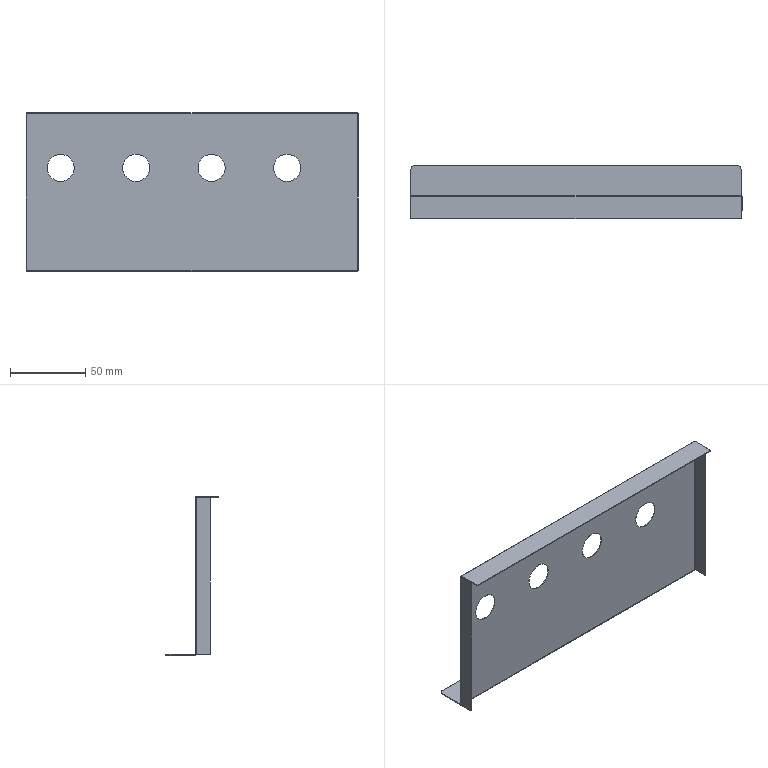Part | SolidWorks | features EdgeFlange 1, Fillet 1, FlatPattern 1, ICE 1, SMBaseFlange 1, SheetMetal 1 | 1 solid | 48 faces | box 220 x 35.5 x 105 mm | volume 15806 mm3 | plane 26 | cylinder 18 | spline 4 | commonest cylinder face diameters 18 x8 0.2 x4 1.2 x4 5 x2
STEP:
#1=CARTESIAN_POINT('',(23.,0.,59.5));
#2=VERTEX_POINT('',#1);
#3=CARTESIAN_POINT('',(23.,0.,77.5));
#4=VERTEX_POINT('',#3);
#5=CARTESIAN_POINT('',(23.,0.,68.5));
#6=DIRECTION('',(0.,1.,0.));
#7=DIRECTION('',(0.,0.,1.));
#8=AXIS2_PLACEMENT_3D('',#5,#6,#7);
#9=CIRCLE('',#8,9.);
#10=EDGE_CURVE('',#2,#4,#9,.T.);
#11=ORIENTED_EDGE('',*,*,#10,.T.);
#12=CARTESIAN_POINT('',(23.,-0.5,77.5));
#13=VERTEX_POINT('',#12);
#14=CARTESIAN_POINT('',(23.,9.5,77.5));
#15=DIRECTION('',(0.,-1.,0.));
#16=VECTOR('',#15,1000.);
#17=LINE('',#14,#16);
#18=EDGE_CURVE('',#4,#13,#17,.T.);
#19=ORIENTED_EDGE('',*,*,#18,.T.);
#20=CARTESIAN_POINT('',(23.,-0.5,59.5));
#21=VERTEX_POINT('',#20);
#22=CARTESIAN_POINT('',(23.,-0.5,68.5));
#23=DIRECTION('',(0.,-1.,0.));
#24=DIRECTION('',(0.,0.,-1.));
#25=AXIS2_PLACEMENT_3D('',#22,#23,#24);
#26=CIRCLE('',#25,9.);
#27=EDGE_CURVE('',#13,#21,#26,.T.);
#28=ORIENTED_EDGE('',*,*,#27,.T.);
#29=CARTESIAN_POINT('',(23.,9.5,59.5));
#30=DIRECTION('',(0.,-1.,0.));
#31=VECTOR('',#30,1000.);
#32=LINE('',#29,#31);
#33=EDGE_CURVE('',#2,#21,#32,.T.);
#34=ORIENTED_EDGE('',*,*,#33,.F.);
#35=EDGE_LOOP('',(#11,#19,#28,#34));
#36=FACE_OUTER_BOUND('',#35,.T.);
#37=CARTESIAN_POINT('',(23.,9.5,68.5));
#38=DIRECTION('',(0.,-1.,0.));
#39=DIRECTION('',(0.,0.,-1.));
#40=AXIS2_PLACEMENT_3D('',#37,#38,#39);
#41=CYLINDRICAL_SURFACE('',#40,9.);
#42=ADVANCED_FACE('',(#36),#41,.F.);
#43=CARTESIAN_POINT('',(73.,0.,59.5));
#44=VERTEX_POINT('',#43);
#45=CARTESIAN_POINT('',(73.,0.,77.5));
#46=VERTEX_POINT('',#45);
#47=CARTESIAN_POINT('',(73.,0.,68.5));
#48=DIRECTION('',(0.,1.,0.));
#49=DIRECTION('',(0.,0.,1.));
#50=AXIS2_PLACEMENT_3D('',#47,#48,#49);
#51=CIRCLE('',#50,9.);
#52=EDGE_CURVE('',#44,#46,#51,.T.);
#53=ORIENTED_EDGE('',*,*,#52,.T.);
#54=CARTESIAN_POINT('',(73.,-0.5,77.5));
#55=VERTEX_POINT('',#54);
#56=CARTESIAN_POINT('',(73.,9.5,77.5));
#57=DIRECTION('',(0.,-1.,0.));
#58=VECTOR('',#57,1000.);
#59=LINE('',#56,#58);
#60=EDGE_CURVE('',#46,#55,#59,.T.);
#61=ORIENTED_EDGE('',*,*,#60,.T.);
#62=CARTESIAN_POINT('',(73.,-0.5,59.5));
#63=VERTEX_POINT('',#62);
#64=CARTESIAN_POINT('',(73.,-0.5,68.5));
#65=DIRECTION('',(0.,-1.,0.));
#66=DIRECTION('',(0.,0.,-1.));
#67=AXIS2_PLACEMENT_3D('',#64,#65,#66);
#68=CIRCLE('',#67,9.);
#69=EDGE_CURVE('',#55,#63,#68,.T.);
#70=ORIENTED_EDGE('',*,*,#69,.T.);
#71=CARTESIAN_POINT('',(73.,9.5,59.5));
#72=DIRECTION('',(0.,-1.,0.));
#73=VECTOR('',#72,1000.);
#74=LINE('',#71,#73);
#75=EDGE_CURVE('',#44,#63,#74,.T.);
#76=ORIENTED_EDGE('',*,*,#75,.F.);
#77=EDGE_LOOP('',(#53,#61,#70,#76));
#78=FACE_OUTER_BOUND('',#77,.T.);
#79=CARTESIAN_POINT('',(73.,9.5,68.5));
#80=DIRECTION('',(0.,-1.,0.));
#81=DIRECTION('',(0.,0.,-1.));
#82=AXIS2_PLACEMENT_3D('',#79,#80,#81);
#83=CYLINDRICAL_SURFACE('',#82,9.);
#84=ADVANCED_FACE('',(#78),#83,.F.);
#85=CARTESIAN_POINT('',(123.,0.,59.5));
#86=VERTEX_POINT('',#85);
#87=CARTESIAN_POINT('',(123.,0.,77.5));
#88=VERTEX_POINT('',#87);
#89=CARTESIAN_POINT('',(123.,0.,68.5));
#90=DIRECTION('',(0.,1.,0.));
#91=DIRECTION('',(0.,0.,1.));
#92=AXIS2_PLACEMENT_3D('',#89,#90,#91);
#93=CIRCLE('',#92,9.);
#94=EDGE_CURVE('',#86,#88,#93,.T.);
#95=ORIENTED_EDGE('',*,*,#94,.T.);
#96=CARTESIAN_POINT('',(123.,-0.5,77.5));
#97=VERTEX_POINT('',#96);
#98=CARTESIAN_POINT('',(123.,9.5,77.5));
#99=DIRECTION('',(0.,-1.,0.));
#100=VECTOR('',#99,1000.);
#101=LINE('',#98,#100);
#102=EDGE_CURVE('',#88,#97,#101,.T.);
#103=ORIENTED_EDGE('',*,*,#102,.T.);
#104=CARTESIAN_POINT('',(123.,-0.5,59.5));
#105=VERTEX_POINT('',#104);
#106=CARTESIAN_POINT('',(123.,-0.5,68.5));
#107=DIRECTION('',(0.,-1.,0.));
#108=DIRECTION('',(0.,0.,-1.));
#109=AXIS2_PLACEMENT_3D('',#106,#107,#108);
#110=CIRCLE('',#109,9.);
#111=EDGE_CURVE('',#97,#105,#110,.T.);
#112=ORIENTED_EDGE('',*,*,#111,.T.);
#113=CARTESIAN_POINT('',(123.,9.5,59.5));
#114=DIRECTION('',(0.,-1.,0.));
#115=VECTOR('',#114,1000.);
#116=LINE('',#113,#115);
#117=EDGE_CURVE('',#86,#105,#116,.T.);
#118=ORIENTED_EDGE('',*,*,#117,.F.);
#119=EDGE_LOOP('',(#95,#103,#112,#118));
#120=FACE_OUTER_BOUND('',#119,.T.);
#121=CARTESIAN_POINT('',(123.,9.5,68.5));
#122=DIRECTION('',(0.,-1.,0.));
#123=DIRECTION('',(0.,0.,-1.));
#124=AXIS2_PLACEMENT_3D('',#121,#122,#123);
#125=CYLINDRICAL_SURFACE('',#124,9.);
#126=ADVANCED_FACE('',(#120),#125,.F.);
#127=CARTESIAN_POINT('',(173.,0.,59.5));
#128=VERTEX_POINT('',#127);
#129=CARTESIAN_POINT('',(173.,0.,77.5));
#130=VERTEX_POINT('',#129);
#131=CARTESIAN_POINT('',(173.,0.,68.5));
#132=DIRECTION('',(0.,1.,0.));
#133=DIRECTION('',(0.,0.,1.));
#134=AXIS2_PLACEMENT_3D('',#131,#132,#133);
#135=CIRCLE('',#134,9.);
#136=EDGE_CURVE('',#128,#130,#135,.T.);
#137=ORIENTED_EDGE('',*,*,#136,.T.);
#138=CARTESIAN_POINT('',(173.,-0.5,77.5));
#139=VERTEX_POINT('',#138);
#140=CARTESIAN_POINT('',(173.,9.5,77.5));
#141=DIRECTION('',(0.,-1.,0.));
#142=VECTOR('',#141,1000.);
#143=LINE('',#140,#142);
#144=EDGE_CURVE('',#130,#139,#143,.T.);
#145=ORIENTED_EDGE('',*,*,#144,.T.);
#146=CARTESIAN_POINT('',(173.,-0.5,59.5));
#147=VERTEX_POINT('',#146);
#148=CARTESIAN_POINT('',(173.,-0.5,68.5));
#149=DIRECTION('',(0.,-1.,0.));
#150=DIRECTION('',(0.,0.,-1.));
#151=AXIS2_PLACEMENT_3D('',#148,#149,#150);
#152=CIRCLE('',#151,9.);
#153=EDGE_CURVE('',#139,#147,#152,.T.);
#154=ORIENTED_EDGE('',*,*,#153,.T.);
#155=CARTESIAN_POINT('',(173.,9.5,59.5));
#156=DIRECTION('',(0.,-1.,0.));
#157=VECTOR('',#156,1000.);
#158=LINE('',#155,#157);
#159=EDGE_CURVE('',#128,#147,#158,.T.);
#160=ORIENTED_EDGE('',*,*,#159,.F.);
#161=EDGE_LOOP('',(#137,#145,#154,#160));
#162=FACE_OUTER_BOUND('',#161,.T.);
#163=CARTESIAN_POINT('',(173.,9.5,68.5));
#164=DIRECTION('',(0.,-1.,0.));
#165=DIRECTION('',(0.,0.,-1.));
#166=AXIS2_PLACEMENT_3D('',#163,#164,#165);
#167=CYLINDRICAL_SURFACE('',#166,9.);
#168=ADVANCED_FACE('',(#162),#167,.F.);
#169=CARTESIAN_POINT('',(23.,-0.5,68.5));
#170=DIRECTION('',(0.,-1.,0.));
#171=DIRECTION('',(0.,0.,-1.));
#172=AXIS2_PLACEMENT_3D('',#169,#170,#171);
#173=CIRCLE('',#172,9.);
#174=EDGE_CURVE('',#21,#13,#173,.T.);
#175=ORIENTED_EDGE('',*,*,#174,.F.);
#176=ORIENTED_EDGE('',*,*,#27,.F.);
#177=EDGE_LOOP('',(#175,#176));
#178=FACE_BOUND('',#177,.T.);
#179=CARTESIAN_POINT('',(73.,-0.5,68.5));
#180=DIRECTION('',(0.,-1.,0.));
#181=DIRECTION('',(0.,0.,-1.));
#182=AXIS2_PLACEMENT_3D('',#179,#180,#181);
#183=CIRCLE('',#182,9.);
#184=EDGE_CURVE('',#63,#55,#183,.T.);
#185=ORIENTED_EDGE('',*,*,#184,.F.);
#186=ORIENTED_EDGE('',*,*,#69,.F.);
#187=EDGE_LOOP('',(#185,#186));
#188=FACE_BOUND('',#187,.T.);
#189=CARTESIAN_POINT('',(123.,-0.5,68.5));
#190=DIRECTION('',(0.,-1.,0.));
#191=DIRECTION('',(0.,0.,-1.));
#192=AXIS2_PLACEMENT_3D('',#189,#190,#191);
#193=CIRCLE('',#192,9.);
#194=EDGE_CURVE('',#105,#97,#193,.T.);
#195=ORIENTED_EDGE('',*,*,#194,.F.);
#196=ORIENTED_EDGE('',*,*,#111,.F.);
#197=EDGE_LOOP('',(#195,#196));
#198=FACE_BOUND('',#197,.T.);
#199=CARTESIAN_POINT('',(173.,-0.5,68.5));
#200=DIRECTION('',(0.,-1.,0.));
#201=DIRECTION('',(0.,0.,-1.));
#202=AXIS2_PLACEMENT_3D('',#199,#200,#201);
#203=CIRCLE('',#202,9.);
#204=EDGE_CURVE('',#147,#139,#203,.T.);
#205=ORIENTED_EDGE('',*,*,#204,.F.);
#206=ORIENTED_EDGE('',*,*,#153,.F.);
#207=EDGE_LOOP('',(#205,#206));
#208=FACE_BOUND('',#207,.T.);
#209=CARTESIAN_POINT('',(219.4,-0.5,104.4));
#210=VERTEX_POINT('',#209);
#211=CARTESIAN_POINT('',(219.4,-0.5,0.6));
#212=VERTEX_POINT('',#211);
#213=CARTESIAN_POINT('',(219.4,-0.5,104.429));
#214=DIRECTION('',(0.,0.,-1.));
#215=VECTOR('',#214,1000.);
#216=LINE('',#213,#215);
#217=EDGE_CURVE('',#210,#212,#216,.T.);
#218=ORIENTED_EDGE('',*,*,#217,.F.);
#219=CARTESIAN_POINT('',(0.6,-0.5,104.4));
#220=VERTEX_POINT('',#219);
#221=CARTESIAN_POINT('',(0.5707,-0.5,104.4));
#222=DIRECTION('',(1.,0.,0.));
#223=VECTOR('',#222,1000.);
#224=LINE('',#221,#223);
#225=EDGE_CURVE('',#220,#210,#224,.T.);
#226=ORIENTED_EDGE('',*,*,#225,.F.);
#227=CARTESIAN_POINT('',(0.6,-0.5,0.6));
#228=VERTEX_POINT('',#227);
#229=CARTESIAN_POINT('',(0.6,-0.5,0.6));
#230=DIRECTION('',(0.,0.,1.));
#231=VECTOR('',#230,1000.);
#232=LINE('',#229,#231);
#233=EDGE_CURVE('',#228,#220,#232,.T.);
#234=ORIENTED_EDGE('',*,*,#233,.F.);
#235=CARTESIAN_POINT('',(0.6,-0.5,0.6));
#236=DIRECTION('',(1.,0.,0.));
#237=VECTOR('',#236,1000.);
#238=LINE('',#235,#237);
#239=EDGE_CURVE('',#228,#212,#238,.T.);
#240=ORIENTED_EDGE('',*,*,#239,.T.);
#241=EDGE_LOOP('',(#218,#226,#234,#240));
#242=FACE_OUTER_BOUND('',#241,.T.);
#243=CARTESIAN_POINT('',(0.,-0.5,105.));
#244=DIRECTION('',(0.,1.,0.));
#245=DIRECTION('',(0.,0.,1.));
#246=AXIS2_PLACEMENT_3D('',#243,#244,#245);
#247=PLANE('',#246);
#248=ADVANCED_FACE('',(#178,#188,#198,#208,#242),#247,.F.);
#249=ORIENTED_EDGE('',*,*,#10,.F.);
#250=CARTESIAN_POINT('',(23.,0.,68.5));
#251=DIRECTION('',(0.,1.,0.));
#252=DIRECTION('',(0.,0.,1.));
#253=AXIS2_PLACEMENT_3D('',#250,#251,#252);
#254=CIRCLE('',#253,9.);
#255=EDGE_CURVE('',#4,#2,#254,.T.);
#256=ORIENTED_EDGE('',*,*,#255,.F.);
#257=EDGE_LOOP('',(#249,#256));
#258=FACE_BOUND('',#257,.T.);
#259=ORIENTED_EDGE('',*,*,#52,.F.);
#260=CARTESIAN_POINT('',(73.,0.,68.5));
#261=DIRECTION('',(0.,1.,0.));
#262=DIRECTION('',(0.,0.,1.));
#263=AXIS2_PLACEMENT_3D('',#260,#261,#262);
#264=CIRCLE('',#263,9.);
#265=EDGE_CURVE('',#46,#44,#264,.T.);
#266=ORIENTED_EDGE('',*,*,#265,.F.);
#267=EDGE_LOOP('',(#259,#266));
#268=FACE_BOUND('',#267,.T.);
#269=ORIENTED_EDGE('',*,*,#94,.F.);
#270=CARTESIAN_POINT('',(123.,0.,68.5));
#271=DIRECTION('',(0.,1.,0.));
#272=DIRECTION('',(0.,0.,1.));
#273=AXIS2_PLACEMENT_3D('',#270,#271,#272);
#274=CIRCLE('',#273,9.);
#275=EDGE_CURVE('',#88,#86,#274,.T.);
#276=ORIENTED_EDGE('',*,*,#275,.F.);
#277=EDGE_LOOP('',(#269,#276));
#278=FACE_BOUND('',#277,.T.);
#279=ORIENTED_EDGE('',*,*,#136,.F.);
#280=CARTESIAN_POINT('',(173.,0.,68.5));
#281=DIRECTION('',(0.,1.,0.));
#282=DIRECTION('',(0.,0.,1.));
#283=AXIS2_PLACEMENT_3D('',#280,#281,#282);
#284=CIRCLE('',#283,9.);
#285=EDGE_CURVE('',#130,#128,#284,.T.);
#286=ORIENTED_EDGE('',*,*,#285,.F.);
#287=EDGE_LOOP('',(#279,#286));
#288=FACE_BOUND('',#287,.T.);
#289=CARTESIAN_POINT('',(0.6,0.,104.4));
#290=VERTEX_POINT('',#289);
#291=CARTESIAN_POINT('',(219.4,0.,104.4));
#292=VERTEX_POINT('',#291);
#293=CARTESIAN_POINT('',(0.5707,0.,104.4));
#294=DIRECTION('',(1.,0.,0.));
#295=VECTOR('',#294,1000.);
#296=LINE('',#293,#295);
#297=EDGE_CURVE('',#290,#292,#296,.T.);
#298=ORIENTED_EDGE('',*,*,#297,.T.);
#299=CARTESIAN_POINT('',(219.4,0.,0.6));
#300=VERTEX_POINT('',#299);
#301=CARTESIAN_POINT('',(219.4,0.,104.429));
#302=DIRECTION('',(0.,0.,-1.));
#303=VECTOR('',#302,1000.);
#304=LINE('',#301,#303);
#305=EDGE_CURVE('',#292,#300,#304,.T.);
#306=ORIENTED_EDGE('',*,*,#305,.T.);
#307=CARTESIAN_POINT('',(0.6,0.,0.6));
#308=VERTEX_POINT('',#307);
#309=CARTESIAN_POINT('',(0.6,0.,0.6));
#310=DIRECTION('',(1.,0.,0.));
#311=VECTOR('',#310,1000.);
#312=LINE('',#309,#311);
#313=EDGE_CURVE('',#308,#300,#312,.T.);
#314=ORIENTED_EDGE('',*,*,#313,.F.);
#315=CARTESIAN_POINT('',(0.6,0.,0.6));
#316=DIRECTION('',(0.,0.,1.));
#317=VECTOR('',#316,1000.);
#318=LINE('',#315,#317);
#319=EDGE_CURVE('',#308,#290,#318,.T.);
#320=ORIENTED_EDGE('',*,*,#319,.T.);
#321=EDGE_LOOP('',(#298,#306,#314,#320));
#322=FACE_OUTER_BOUND('',#321,.T.);
#323=CARTESIAN_POINT('',(0.,0.,105.));
#324=DIRECTION('',(0.,1.,0.));
#325=DIRECTION('',(0.,0.,1.));
#326=AXIS2_PLACEMENT_3D('',#323,#324,#325);
#327=PLANE('',#326);
#328=ADVANCED_FACE('',(#258,#268,#278,#288,#322),#327,.T.);
#329=CARTESIAN_POINT('',(0.,-0.6,104.429));
#330=VERTEX_POINT('',#329);
#331=CARTESIAN_POINT('',(0.5,-0.6,104.429));
#332=VERTEX_POINT('',#331);
#333=CARTESIAN_POINT('',(0.5,-0.6,104.429));
#334=DIRECTION('',(1.,0.,0.));
#335=VECTOR('',#334,1000.);
#336=LINE('',#333,#335);
#337=EDGE_CURVE('',#330,#332,#336,.T.);
#338=ORIENTED_EDGE('',*,*,#337,.T.);
#339=CARTESIAN_POINT('',(0.6,-0.5,104.4));
#340=CARTESIAN_POINT('',(0.5738,-0.5,104.405));
#341=CARTESIAN_POINT('',(0.5478,-0.5108,104.41));
#342=CARTESIAN_POINT('',(0.5108,-0.5478,104.42));
#343=CARTESIAN_POINT('',(0.5,-0.5738,104.424));
#344=CARTESIAN_POINT('',(0.5,-0.6,104.429));
#345=B_SPLINE_CURVE_WITH_KNOTS('',3,(#339,#340,#341,#342,#343,#344),.UNSPECIFIED.,.F.,.F.,(4,2,4),(0.,0.5,1.),.UNSPECIFIED.);
#346=EDGE_CURVE('',#220,#332,#345,.T.);
#347=ORIENTED_EDGE('',*,*,#346,.F.);
#348=CARTESIAN_POINT('',(0.6,-0.5,104.4));
#349=DIRECTION('',(0.,1.,0.));
#350=VECTOR('',#349,1000.);
#351=LINE('',#348,#350);
#352=EDGE_CURVE('',#220,#290,#351,.T.);
#353=ORIENTED_EDGE('',*,*,#352,.T.);
#354=CARTESIAN_POINT('',(0.6,0.,104.4));
#355=CARTESIAN_POINT('',(0.4429,0.,104.405));
#356=CARTESIAN_POINT('',(0.2868,-0.06466,104.41));
#357=CARTESIAN_POINT('',(0.06466,-0.2868,104.42));
#358=CARTESIAN_POINT('',(0.,-0.4429,104.424));
#359=CARTESIAN_POINT('',(0.,-0.6,104.429));
#360=B_SPLINE_CURVE_WITH_KNOTS('',3,(#354,#355,#356,#357,#358,#359),.UNSPECIFIED.,.F.,.F.,(4,2,4),(0.,0.5,1.),.UNSPECIFIED.);
#361=EDGE_CURVE('',#290,#330,#360,.T.);
#362=ORIENTED_EDGE('',*,*,#361,.T.);
#363=EDGE_LOOP('',(#338,#347,#353,#362));
#364=FACE_OUTER_BOUND('',#363,.T.);
#365=CARTESIAN_POINT('',(0.6,0.005,104.4));
#366=CARTESIAN_POINT('',(0.5208,0.005,104.402));
#367=CARTESIAN_POINT('',(0.4416,-0.01075,104.405));
#368=CARTESIAN_POINT('',(0.2953,-0.07136,104.41));
#369=CARTESIAN_POINT('',(0.2282,-0.1162,104.412));
#370=CARTESIAN_POINT('',(0.1162,-0.2282,104.417));
#371=CARTESIAN_POINT('',(0.07136,-0.2953,104.42));
#372=CARTESIAN_POINT('',(0.01075,-0.4416,104.424));
#373=CARTESIAN_POINT('',(-0.005,-0.5208,104.427));
#374=CARTESIAN_POINT('',(-0.005,-0.6,104.429));
#375=CARTESIAN_POINT('',(0.6,0.,104.4));
#376=CARTESIAN_POINT('',(0.5214,0.,104.402));
#377=CARTESIAN_POINT('',(0.443,-0.01562,104.405));
#378=CARTESIAN_POINT('',(0.2978,-0.07573,104.41));
#379=CARTESIAN_POINT('',(0.2313,-0.1202,104.412));
#380=CARTESIAN_POINT('',(0.1202,-0.2313,104.417));
#381=CARTESIAN_POINT('',(0.07573,-0.2978,104.42));
#382=CARTESIAN_POINT('',(0.01562,-0.443,104.424));
#383=CARTESIAN_POINT('',(0.,-0.5214,104.427));
#384=CARTESIAN_POINT('',(0.,-0.6,104.429));
#385=CARTESIAN_POINT('',(0.6,-0.5,104.4));
#386=CARTESIAN_POINT('',(0.5869,-0.5,104.402));
#387=CARTESIAN_POINT('',(0.5738,-0.5026,104.405));
#388=CARTESIAN_POINT('',(0.5496,-0.5126,104.41));
#389=CARTESIAN_POINT('',(0.5385,-0.52,104.412));
#390=CARTESIAN_POINT('',(0.52,-0.5385,104.417));
#391=CARTESIAN_POINT('',(0.5126,-0.5496,104.42));
#392=CARTESIAN_POINT('',(0.5026,-0.5738,104.424));
#393=CARTESIAN_POINT('',(0.5,-0.5869,104.427));
#394=CARTESIAN_POINT('',(0.5,-0.6,104.429));
#395=CARTESIAN_POINT('',(0.6,-0.505,104.4));
#396=CARTESIAN_POINT('',(0.5876,-0.505,104.402));
#397=CARTESIAN_POINT('',(0.5751,-0.5075,104.405));
#398=CARTESIAN_POINT('',(0.5522,-0.517,104.41));
#399=CARTESIAN_POINT('',(0.5416,-0.5241,104.412));
#400=CARTESIAN_POINT('',(0.5241,-0.5416,104.417));
#401=CARTESIAN_POINT('',(0.517,-0.5522,104.42));
#402=CARTESIAN_POINT('',(0.5075,-0.5751,104.424));
#403=CARTESIAN_POINT('',(0.505,-0.5876,104.427));
#404=CARTESIAN_POINT('',(0.505,-0.6,104.429));
#405=B_SPLINE_SURFACE_WITH_KNOTS('',1,3,((#365,#366,#367,#368,#369,#370,#371,#372,#373,#374),(#375,#376,#377,#378,#379,#380,#381,#382,#383,#384),(#385,#386,#387,#388,#389,#390,#391,#392,#393,#394),(#395,#396,#397,#398,#399,#400,#401,#402,#403,#404)),.UNSPECIFIED.,.F.,.F.,.F.,(2,1,1,2),(4,2,2,2,4),(-0.01,0.,1.,1.01),(0.,0.25,0.5,0.75,1.),.UNSPECIFIED.);
#406=ADVANCED_FACE('',(#364),#405,.F.);
#407=ORIENTED_EDGE('',*,*,#319,.F.);
#408=CARTESIAN_POINT('',(0.,-0.6,0.6));
#409=VERTEX_POINT('',#408);
#410=CARTESIAN_POINT('',(0.6,-0.6,0.6));
#411=DIRECTION('',(0.,0.,-1.));
#412=DIRECTION('',(-1.,0.,0.));
#413=AXIS2_PLACEMENT_3D('',#410,#411,#412);
#414=CIRCLE('',#413,0.6);
#415=EDGE_CURVE('',#409,#308,#414,.T.);
#416=ORIENTED_EDGE('',*,*,#415,.F.);
#417=CARTESIAN_POINT('',(0.,-0.6,0.));
#418=DIRECTION('',(0.,0.,-1.));
#419=VECTOR('',#418,1000.);
#420=LINE('',#417,#419);
#421=EDGE_CURVE('',#330,#409,#420,.T.);
#422=ORIENTED_EDGE('',*,*,#421,.F.);
#423=ORIENTED_EDGE('',*,*,#361,.F.);
#424=EDGE_LOOP('',(#407,#416,#422,#423));
#425=FACE_OUTER_BOUND('',#424,.T.);
#426=CARTESIAN_POINT('',(0.6,-0.6,0.6));
#427=DIRECTION('',(0.,0.,-1.));
#428=DIRECTION('',(-1.,0.,0.));
#429=AXIS2_PLACEMENT_3D('',#426,#427,#428);
#430=CYLINDRICAL_SURFACE('',#429,0.6);
#431=ADVANCED_FACE('',(#425),#430,.T.);
#432=CARTESIAN_POINT('',(0.5,-0.6,0.6));
#433=VERTEX_POINT('',#432);
#434=CARTESIAN_POINT('',(0.6,-0.6,0.6));
#435=DIRECTION('',(0.,0.,-1.));
#436=DIRECTION('',(-1.,0.,0.));
#437=AXIS2_PLACEMENT_3D('',#434,#435,#436);
#438=CIRCLE('',#437,0.1);
#439=EDGE_CURVE('',#433,#228,#438,.T.);
#440=ORIENTED_EDGE('',*,*,#439,.F.);
#441=CARTESIAN_POINT('',(0.5,-0.6,0.6));
#442=DIRECTION('',(1.,0.,0.));
#443=VECTOR('',#442,1000.);
#444=LINE('',#441,#443);
#445=EDGE_CURVE('',#409,#433,#444,.T.);
#446=ORIENTED_EDGE('',*,*,#445,.F.);
#447=ORIENTED_EDGE('',*,*,#415,.T.);
#448=CARTESIAN_POINT('',(0.6,-0.5,0.6));
#449=DIRECTION('',(0.,1.,0.));
#450=VECTOR('',#449,1000.);
#451=LINE('',#448,#450);
#452=EDGE_CURVE('',#228,#308,#451,.T.);
#453=ORIENTED_EDGE('',*,*,#452,.F.);
#454=EDGE_LOOP('',(#440,#446,#447,#453));
#455=FACE_OUTER_BOUND('',#454,.T.);
#456=CARTESIAN_POINT('',(0.6,-0.6,0.6));
#457=DIRECTION('',(0.,0.,1.));
#458=DIRECTION('',(1.,0.,0.));
#459=AXIS2_PLACEMENT_3D('',#456,#457,#458);
#460=PLANE('',#459);
#461=ADVANCED_FACE('',(#455),#460,.F.);
#462=ORIENTED_EDGE('',*,*,#233,.T.);
#463=ORIENTED_EDGE('',*,*,#346,.T.);
#464=CARTESIAN_POINT('',(0.5,-0.6,105.));
#465=DIRECTION('',(0.,0.,-1.));
#466=VECTOR('',#465,1000.);
#467=LINE('',#464,#466);
#468=EDGE_CURVE('',#332,#433,#467,.T.);
#469=ORIENTED_EDGE('',*,*,#468,.T.);
#470=ORIENTED_EDGE('',*,*,#439,.T.);
#471=EDGE_LOOP('',(#462,#463,#469,#470));
#472=FACE_OUTER_BOUND('',#471,.T.);
#473=CARTESIAN_POINT('',(0.6,-0.6,0.6));
#474=DIRECTION('',(0.,0.,-1.));
#475=DIRECTION('',(-1.,0.,0.));
#476=AXIS2_PLACEMENT_3D('',#473,#474,#475);
#477=CYLINDRICAL_SURFACE('',#476,0.1);
#478=ADVANCED_FACE('',(#472),#477,.F.);
#479=CARTESIAN_POINT('',(0.5,-10.,104.429));
#480=VERTEX_POINT('',#479);
#481=CARTESIAN_POINT('',(0.,-10.,104.429));
#482=VERTEX_POINT('',#481);
#483=CARTESIAN_POINT('',(0.,-10.,104.429));
#484=DIRECTION('',(-1.,0.,0.));
#485=VECTOR('',#484,1000.);
#486=LINE('',#483,#485);
#487=EDGE_CURVE('',#480,#482,#486,.T.);
#488=ORIENTED_EDGE('',*,*,#487,.F.);
#489=CARTESIAN_POINT('',(0.5,-0.5,104.429));
#490=DIRECTION('',(0.,-1.,0.));
#491=VECTOR('',#490,1000.);
#492=LINE('',#489,#491);
#493=EDGE_CURVE('',#332,#480,#492,.T.);
#494=ORIENTED_EDGE('',*,*,#493,.F.);
#495=ORIENTED_EDGE('',*,*,#337,.F.);
#496=CARTESIAN_POINT('',(0.,-0.5,104.429));
#497=DIRECTION('',(0.,1.,0.));
#498=VECTOR('',#497,1000.);
#499=LINE('',#496,#498);
#500=EDGE_CURVE('',#482,#330,#499,.T.);
#501=ORIENTED_EDGE('',*,*,#500,.F.);
#502=EDGE_LOOP('',(#488,#494,#495,#501));
#503=FACE_OUTER_BOUND('',#502,.T.);
#504=CARTESIAN_POINT('',(0.5,-0.5,104.429));
#505=DIRECTION('',(0.,0.,1.));
#506=DIRECTION('',(0.,-1.,0.));
#507=AXIS2_PLACEMENT_3D('',#504,#505,#506);
#508=PLANE('',#507);
#509=ADVANCED_FACE('',(#503),#508,.T.);
#510=CARTESIAN_POINT('',(0.,-10.,0.6));
#511=VERTEX_POINT('',#510);
#512=CARTESIAN_POINT('',(0.,-0.5,0.6));
#513=DIRECTION('',(0.,1.,0.));
#514=VECTOR('',#513,1000.);
#515=LINE('',#512,#514);
#516=EDGE_CURVE('',#511,#409,#515,.T.);
#517=ORIENTED_EDGE('',*,*,#516,.F.);
#518=CARTESIAN_POINT('',(0.,-10.,0.));
#519=DIRECTION('',(0.,0.,-1.));
#520=VECTOR('',#519,1000.);
#521=LINE('',#518,#520);
#522=EDGE_CURVE('',#482,#511,#521,.T.);
#523=ORIENTED_EDGE('',*,*,#522,.F.);
#524=ORIENTED_EDGE('',*,*,#500,.T.);
#525=ORIENTED_EDGE('',*,*,#421,.T.);
#526=EDGE_LOOP('',(#517,#523,#524,#525));
#527=FACE_OUTER_BOUND('',#526,.T.);
#528=CARTESIAN_POINT('',(0.,-0.5,0.));
#529=DIRECTION('',(-1.,0.,0.));
#530=DIRECTION('',(0.,-1.,0.));
#531=AXIS2_PLACEMENT_3D('',#528,#529,#530);
#532=PLANE('',#531);
#533=ADVANCED_FACE('',(#527),#532,.T.);
#534=CARTESIAN_POINT('',(0.5,-10.,0.6));
#535=VERTEX_POINT('',#534);
#536=CARTESIAN_POINT('',(0.5,-10.,0.));
#537=DIRECTION('',(0.,0.,-1.));
#538=VECTOR('',#537,1000.);
#539=LINE('',#536,#538);
#540=EDGE_CURVE('',#480,#535,#539,.T.);
#541=ORIENTED_EDGE('',*,*,#540,.T.);
#542=CARTESIAN_POINT('',(0.5,-0.5,0.6));
#543=DIRECTION('',(0.,-1.,0.));
#544=VECTOR('',#543,1000.);
#545=LINE('',#542,#544);
#546=EDGE_CURVE('',#433,#535,#545,.T.);
#547=ORIENTED_EDGE('',*,*,#546,.F.);
#548=ORIENTED_EDGE('',*,*,#468,.F.);
#549=ORIENTED_EDGE('',*,*,#493,.T.);
#550=EDGE_LOOP('',(#541,#547,#548,#549));
#551=FACE_OUTER_BOUND('',#550,.T.);
#552=CARTESIAN_POINT('',(0.5,-0.5,0.));
#553=DIRECTION('',(-1.,0.,0.));
#554=DIRECTION('',(0.,-1.,0.));
#555=AXIS2_PLACEMENT_3D('',#552,#553,#554);
#556=PLANE('',#555);
#557=ADVANCED_FACE('',(#551),#556,.F.);
#558=CARTESIAN_POINT('',(0.5,-10.,0.6));
#559=DIRECTION('',(-1.,0.,0.));
#560=VECTOR('',#559,1000.);
#561=LINE('',#558,#560);
#562=EDGE_CURVE('',#535,#511,#561,.T.);
#563=ORIENTED_EDGE('',*,*,#562,.F.);
#564=ORIENTED_EDGE('',*,*,#540,.F.);
#565=ORIENTED_EDGE('',*,*,#487,.T.);
#566=ORIENTED_EDGE('',*,*,#522,.T.);
#567=EDGE_LOOP('',(#563,#564,#565,#566));
#568=FACE_OUTER_BOUND('',#567,.T.);
#569=CARTESIAN_POINT('',(0.,-10.,0.));
#570=DIRECTION('',(0.,-1.,0.));
#571=DIRECTION('',(1.,0.,0.));
#572=AXIS2_PLACEMENT_3D('',#569,#570,#571);
#573=PLANE('',#572);
#574=ADVANCED_FACE('',(#568),#573,.T.);
#575=ORIENTED_EDGE('',*,*,#546,.T.);
#576=ORIENTED_EDGE('',*,*,#562,.T.);
#577=ORIENTED_EDGE('',*,*,#516,.T.);
#578=ORIENTED_EDGE('',*,*,#445,.T.);
#579=EDGE_LOOP('',(#575,#576,#577,#578));
#580=FACE_OUTER_BOUND('',#579,.T.);
#581=CARTESIAN_POINT('',(0.5,-0.5,0.6));
#582=DIRECTION('',(0.,0.,1.));
#583=DIRECTION('',(0.,-1.,0.));
#584=AXIS2_PLACEMENT_3D('',#581,#582,#583);
#585=PLANE('',#584);
#586=ADVANCED_FACE('',(#580),#585,.F.);
#587=CARTESIAN_POINT('',(219.429,-0.6,105.));
#588=VERTEX_POINT('',#587);
#589=CARTESIAN_POINT('',(219.429,-0.6,104.5));
#590=VERTEX_POINT('',#589);
#591=CARTESIAN_POINT('',(219.429,-0.6,104.5));
#592=DIRECTION('',(0.,0.,-1.));
#593=VECTOR('',#592,1000.);
#594=LINE('',#591,#593);
#595=EDGE_CURVE('',#588,#590,#594,.T.);
#596=ORIENTED_EDGE('',*,*,#595,.T.);
#597=CARTESIAN_POINT('',(219.4,-0.5,104.4));
#598=CARTESIAN_POINT('',(219.405,-0.5,104.426));
#599=CARTESIAN_POINT('',(219.41,-0.5108,104.452));
#600=CARTESIAN_POINT('',(219.42,-0.5478,104.489));
#601=CARTESIAN_POINT('',(219.424,-0.5738,104.5));
#602=CARTESIAN_POINT('',(219.429,-0.6,104.5));
#603=B_SPLINE_CURVE_WITH_KNOTS('',3,(#597,#598,#599,#600,#601,#602),.UNSPECIFIED.,.F.,.F.,(4,2,4),(0.,0.5,1.),.UNSPECIFIED.);
#604=EDGE_CURVE('',#210,#590,#603,.T.);
#605=ORIENTED_EDGE('',*,*,#604,.F.);
#606=CARTESIAN_POINT('',(219.4,-0.5,104.4));
#607=DIRECTION('',(0.,1.,0.));
#608=VECTOR('',#607,1000.);
#609=LINE('',#606,#608);
#610=EDGE_CURVE('',#210,#292,#609,.T.);
#611=ORIENTED_EDGE('',*,*,#610,.T.);
#612=CARTESIAN_POINT('',(219.4,0.,104.4));
#613=CARTESIAN_POINT('',(219.405,0.,104.557));
#614=CARTESIAN_POINT('',(219.41,-0.06466,104.713));
#615=CARTESIAN_POINT('',(219.42,-0.2868,104.935));
#616=CARTESIAN_POINT('',(219.424,-0.4429,105.));
#617=CARTESIAN_POINT('',(219.429,-0.6,105.));
#618=B_SPLINE_CURVE_WITH_KNOTS('',3,(#612,#613,#614,#615,#616,#617),.UNSPECIFIED.,.F.,.F.,(4,2,4),(0.,0.5,1.),.UNSPECIFIED.);
#619=EDGE_CURVE('',#292,#588,#618,.T.);
#620=ORIENTED_EDGE('',*,*,#619,.T.);
#621=EDGE_LOOP('',(#596,#605,#611,#620));
#622=FACE_OUTER_BOUND('',#621,.T.);
#623=CARTESIAN_POINT('',(219.4,0.005,104.4));
#624=CARTESIAN_POINT('',(219.402,0.005,104.479));
#625=CARTESIAN_POINT('',(219.405,-0.01075,104.558));
#626=CARTESIAN_POINT('',(219.41,-0.07136,104.705));
#627=CARTESIAN_POINT('',(219.412,-0.1162,104.772));
#628=CARTESIAN_POINT('',(219.417,-0.2282,104.884));
#629=CARTESIAN_POINT('',(219.42,-0.2953,104.929));
#630=CARTESIAN_POINT('',(219.424,-0.4416,104.989));
#631=CARTESIAN_POINT('',(219.427,-0.5208,105.005));
#632=CARTESIAN_POINT('',(219.429,-0.6,105.005));
#633=CARTESIAN_POINT('',(219.4,0.,104.4));
#634=CARTESIAN_POINT('',(219.402,0.,104.479));
#635=CARTESIAN_POINT('',(219.405,-0.01562,104.557));
#636=CARTESIAN_POINT('',(219.41,-0.07573,104.702));
#637=CARTESIAN_POINT('',(219.412,-0.1202,104.769));
#638=CARTESIAN_POINT('',(219.417,-0.2313,104.88));
#639=CARTESIAN_POINT('',(219.42,-0.2978,104.924));
#640=CARTESIAN_POINT('',(219.424,-0.443,104.984));
#641=CARTESIAN_POINT('',(219.427,-0.5214,105.));
#642=CARTESIAN_POINT('',(219.429,-0.6,105.));
#643=CARTESIAN_POINT('',(219.4,-0.5,104.4));
#644=CARTESIAN_POINT('',(219.402,-0.5,104.413));
#645=CARTESIAN_POINT('',(219.405,-0.5026,104.426));
#646=CARTESIAN_POINT('',(219.41,-0.5126,104.45));
#647=CARTESIAN_POINT('',(219.412,-0.52,104.461));
#648=CARTESIAN_POINT('',(219.417,-0.5385,104.48));
#649=CARTESIAN_POINT('',(219.42,-0.5496,104.487));
#650=CARTESIAN_POINT('',(219.424,-0.5738,104.497));
#651=CARTESIAN_POINT('',(219.427,-0.5869,104.5));
#652=CARTESIAN_POINT('',(219.429,-0.6,104.5));
#653=CARTESIAN_POINT('',(219.4,-0.5051,104.4));
#654=CARTESIAN_POINT('',(219.402,-0.5051,104.412));
#655=CARTESIAN_POINT('',(219.405,-0.5075,104.425));
#656=CARTESIAN_POINT('',(219.41,-0.517,104.448));
#657=CARTESIAN_POINT('',(219.412,-0.5241,104.458));
#658=CARTESIAN_POINT('',(219.417,-0.5416,104.476));
#659=CARTESIAN_POINT('',(219.42,-0.5522,104.483));
#660=CARTESIAN_POINT('',(219.424,-0.5751,104.492));
#661=CARTESIAN_POINT('',(219.427,-0.5876,104.495));
#662=CARTESIAN_POINT('',(219.429,-0.6,104.495));
#663=B_SPLINE_SURFACE_WITH_KNOTS('',1,3,((#623,#624,#625,#626,#627,#628,#629,#630,#631,#632),(#633,#634,#635,#636,#637,#638,#639,#640,#641,#642),(#643,#644,#645,#646,#647,#648,#649,#650,#651,#652),(#653,#654,#655,#656,#657,#658,#659,#660,#661,#662)),.UNSPECIFIED.,.F.,.F.,.F.,(2,1,1,2),(4,2,2,2,4),(-0.01,0.,1.,1.01),(0.,0.25,0.5,0.75,1.),.UNSPECIFIED.);
#664=ADVANCED_FACE('',(#622),#663,.F.);
#665=ORIENTED_EDGE('',*,*,#297,.F.);
#666=CARTESIAN_POINT('',(0.5707,-0.6,105.));
#667=VERTEX_POINT('',#666);
#668=CARTESIAN_POINT('',(0.5707,-0.6,105.));
#669=CARTESIAN_POINT('',(0.5756,-0.4429,105.));
#670=CARTESIAN_POINT('',(0.5805,-0.2868,104.935));
#671=CARTESIAN_POINT('',(0.5902,-0.06466,104.713));
#672=CARTESIAN_POINT('',(0.5951,0.,104.557));
#673=CARTESIAN_POINT('',(0.6,0.,104.4));
#674=B_SPLINE_CURVE_WITH_KNOTS('',3,(#668,#669,#670,#671,#672,#673),.UNSPECIFIED.,.F.,.F.,(4,2,4),(0.,0.5,1.),.UNSPECIFIED.);
#675=EDGE_CURVE('',#667,#290,#674,.T.);
#676=ORIENTED_EDGE('',*,*,#675,.F.);
#677=CARTESIAN_POINT('',(220.,-0.6,105.));
#678=DIRECTION('',(1.,0.,0.));
#679=VECTOR('',#678,1000.);
#680=LINE('',#677,#679);
#681=EDGE_CURVE('',#667,#588,#680,.T.);
#682=ORIENTED_EDGE('',*,*,#681,.T.);
#683=ORIENTED_EDGE('',*,*,#619,.F.);
#684=EDGE_LOOP('',(#665,#676,#682,#683));
#685=FACE_OUTER_BOUND('',#684,.T.);
#686=CARTESIAN_POINT('',(0.5707,-0.6,104.4));
#687=DIRECTION('',(-1.,0.,0.));
#688=DIRECTION('',(0.,0.,1.));
#689=AXIS2_PLACEMENT_3D('',#686,#687,#688);
#690=CYLINDRICAL_SURFACE('',#689,0.6);
#691=ADVANCED_FACE('',(#685),#690,.T.);
#692=CARTESIAN_POINT('',(0.5707,-0.6,104.5));
#693=VERTEX_POINT('',#692);
#694=CARTESIAN_POINT('',(0.5707,-0.6,104.5));
#695=CARTESIAN_POINT('',(0.5756,-0.5738,104.5));
#696=CARTESIAN_POINT('',(0.5805,-0.5478,104.489));
#697=CARTESIAN_POINT('',(0.5902,-0.5108,104.452));
#698=CARTESIAN_POINT('',(0.5951,-0.5,104.426));
#699=CARTESIAN_POINT('',(0.6,-0.5,104.4));
#700=B_SPLINE_CURVE_WITH_KNOTS('',3,(#694,#695,#696,#697,#698,#699),.UNSPECIFIED.,.F.,.F.,(4,2,4),(0.,0.5,1.),.UNSPECIFIED.);
#701=EDGE_CURVE('',#693,#220,#700,.T.);
#702=ORIENTED_EDGE('',*,*,#701,.F.);
#703=CARTESIAN_POINT('',(0.5707,-0.6,104.5));
#704=DIRECTION('',(0.,0.,-1.));
#705=VECTOR('',#704,1000.);
#706=LINE('',#703,#705);
#707=EDGE_CURVE('',#667,#693,#706,.T.);
#708=ORIENTED_EDGE('',*,*,#707,.F.);
#709=ORIENTED_EDGE('',*,*,#675,.T.);
#710=ORIENTED_EDGE('',*,*,#352,.F.);
#711=EDGE_LOOP('',(#702,#708,#709,#710));
#712=FACE_OUTER_BOUND('',#711,.T.);
#713=CARTESIAN_POINT('',(0.5707,-0.6,105.005));
#714=CARTESIAN_POINT('',(0.5732,-0.5208,105.005));
#715=CARTESIAN_POINT('',(0.5756,-0.4416,104.989));
#716=CARTESIAN_POINT('',(0.5805,-0.2953,104.929));
#717=CARTESIAN_POINT('',(0.5829,-0.2282,104.884));
#718=CARTESIAN_POINT('',(0.5878,-0.1162,104.772));
#719=CARTESIAN_POINT('',(0.5902,-0.07136,104.705));
#720=CARTESIAN_POINT('',(0.5951,-0.01075,104.558));
#721=CARTESIAN_POINT('',(0.5976,0.005,104.479));
#722=CARTESIAN_POINT('',(0.6,0.005,104.4));
#723=CARTESIAN_POINT('',(0.5707,-0.6,105.));
#724=CARTESIAN_POINT('',(0.5732,-0.5214,105.));
#725=CARTESIAN_POINT('',(0.5756,-0.443,104.984));
#726=CARTESIAN_POINT('',(0.5805,-0.2978,104.924));
#727=CARTESIAN_POINT('',(0.5829,-0.2313,104.88));
#728=CARTESIAN_POINT('',(0.5878,-0.1202,104.769));
#729=CARTESIAN_POINT('',(0.5902,-0.07573,104.702));
#730=CARTESIAN_POINT('',(0.5951,-0.01562,104.557));
#731=CARTESIAN_POINT('',(0.5976,0.,104.479));
#732=CARTESIAN_POINT('',(0.6,0.,104.4));
#733=CARTESIAN_POINT('',(0.5707,-0.6,104.5));
#734=CARTESIAN_POINT('',(0.5732,-0.5869,104.5));
#735=CARTESIAN_POINT('',(0.5756,-0.5738,104.497));
#736=CARTESIAN_POINT('',(0.5805,-0.5496,104.487));
#737=CARTESIAN_POINT('',(0.5829,-0.5385,104.48));
#738=CARTESIAN_POINT('',(0.5878,-0.52,104.461));
#739=CARTESIAN_POINT('',(0.5902,-0.5126,104.45));
#740=CARTESIAN_POINT('',(0.5951,-0.5026,104.426));
#741=CARTESIAN_POINT('',(0.5976,-0.5,104.413));
#742=CARTESIAN_POINT('',(0.6,-0.5,104.4));
#743=CARTESIAN_POINT('',(0.5707,-0.6,104.495));
#744=CARTESIAN_POINT('',(0.5732,-0.5876,104.495));
#745=CARTESIAN_POINT('',(0.5756,-0.5751,104.492));
#746=CARTESIAN_POINT('',(0.5805,-0.5522,104.483));
#747=CARTESIAN_POINT('',(0.5829,-0.5416,104.476));
#748=CARTESIAN_POINT('',(0.5878,-0.5241,104.458));
#749=CARTESIAN_POINT('',(0.5902,-0.517,104.448));
#750=CARTESIAN_POINT('',(0.5951,-0.5075,104.425));
#751=CARTESIAN_POINT('',(0.5976,-0.5051,104.412));
#752=CARTESIAN_POINT('',(0.6,-0.5051,104.4));
#753=B_SPLINE_SURFACE_WITH_KNOTS('',1,3,((#713,#714,#715,#716,#717,#718,#719,#720,#721,#722),(#723,#724,#725,#726,#727,#728,#729,#730,#731,#732),(#733,#734,#735,#736,#737,#738,#739,#740,#741,#742),(#743,#744,#745,#746,#747,#748,#749,#750,#751,#752)),.UNSPECIFIED.,.F.,.F.,.F.,(2,1,1,2),(4,2,2,2,4),(-0.01,0.,1.,1.01),(0.,0.25,0.5,0.75,1.),.UNSPECIFIED.);
#754=ADVANCED_FACE('',(#712),#753,.F.);
#755=ORIENTED_EDGE('',*,*,#225,.T.);
#756=ORIENTED_EDGE('',*,*,#604,.T.);
#757=CARTESIAN_POINT('',(220.,-0.6,104.5));
#758=DIRECTION('',(-1.,0.,0.));
#759=VECTOR('',#758,1000.);
#760=LINE('',#757,#759);
#761=EDGE_CURVE('',#590,#693,#760,.T.);
#762=ORIENTED_EDGE('',*,*,#761,.T.);
#763=ORIENTED_EDGE('',*,*,#701,.T.);
#764=EDGE_LOOP('',(#755,#756,#762,#763));
#765=FACE_OUTER_BOUND('',#764,.T.);
#766=CARTESIAN_POINT('',(0.5707,-0.6,104.4));
#767=DIRECTION('',(-1.,0.,0.));
#768=DIRECTION('',(0.,0.,1.));
#769=AXIS2_PLACEMENT_3D('',#766,#767,#768);
#770=CYLINDRICAL_SURFACE('',#769,0.1);
#771=ADVANCED_FACE('',(#765),#770,.F.);
#772=CARTESIAN_POINT('',(219.429,-15.5,104.5));
#773=VERTEX_POINT('',#772);
#774=CARTESIAN_POINT('',(219.429,-15.5,105.));
#775=VERTEX_POINT('',#774);
#776=CARTESIAN_POINT('',(219.429,-15.5,105.));
#777=DIRECTION('',(0.,0.,1.));
#778=VECTOR('',#777,1000.);
#779=LINE('',#776,#778);
#780=EDGE_CURVE('',#773,#775,#779,.T.);
#781=ORIENTED_EDGE('',*,*,#780,.F.);
#782=CARTESIAN_POINT('',(219.429,-0.5,104.5));
#783=DIRECTION('',(0.,-1.,0.));
#784=VECTOR('',#783,1000.);
#785=LINE('',#782,#784);
#786=EDGE_CURVE('',#590,#773,#785,.T.);
#787=ORIENTED_EDGE('',*,*,#786,.F.);
#788=ORIENTED_EDGE('',*,*,#595,.F.);
#789=CARTESIAN_POINT('',(219.429,-0.5,105.));
#790=DIRECTION('',(0.,-1.,0.));
#791=VECTOR('',#790,1000.);
#792=LINE('',#789,#791);
#793=EDGE_CURVE('',#588,#775,#792,.T.);
#794=ORIENTED_EDGE('',*,*,#793,.T.);
#795=EDGE_LOOP('',(#781,#787,#788,#794));
#796=FACE_OUTER_BOUND('',#795,.T.);
#797=CARTESIAN_POINT('',(219.429,-0.5,104.5));
#798=DIRECTION('',(1.,0.,0.));
#799=DIRECTION('',(0.,0.,-1.));
#800=AXIS2_PLACEMENT_3D('',#797,#798,#799);
#801=PLANE('',#800);
#802=ADVANCED_FACE('',(#796),#801,.T.);
#803=ORIENTED_EDGE('',*,*,#681,.F.);
#804=CARTESIAN_POINT('',(0.5707,-15.5,105.));
#805=VERTEX_POINT('',#804);
#806=CARTESIAN_POINT('',(0.5707,-0.5,105.));
#807=DIRECTION('',(0.,-1.,0.));
#808=VECTOR('',#807,1000.);
#809=LINE('',#806,#808);
#810=EDGE_CURVE('',#667,#805,#809,.T.);
#811=ORIENTED_EDGE('',*,*,#810,.T.);
#812=CARTESIAN_POINT('',(220.,-15.5,105.));
#813=DIRECTION('',(-1.,0.,0.));
#814=VECTOR('',#813,1000.);
#815=LINE('',#812,#814);
#816=EDGE_CURVE('',#775,#805,#815,.T.);
#817=ORIENTED_EDGE('',*,*,#816,.F.);
#818=ORIENTED_EDGE('',*,*,#793,.F.);
#819=EDGE_LOOP('',(#803,#811,#817,#818));
#820=FACE_OUTER_BOUND('',#819,.T.);
#821=CARTESIAN_POINT('',(0.,-0.5,105.));
#822=DIRECTION('',(0.,0.,-1.));
#823=DIRECTION('',(0.,1.,0.));
#824=AXIS2_PLACEMENT_3D('',#821,#822,#823);
#825=PLANE('',#824);
#826=ADVANCED_FACE('',(#820),#825,.F.);
#827=CARTESIAN_POINT('',(0.5707,-15.5,104.5));
#828=VERTEX_POINT('',#827);
#829=CARTESIAN_POINT('',(0.5707,-0.5,104.5));
#830=DIRECTION('',(0.,-1.,0.));
#831=VECTOR('',#830,1000.);
#832=LINE('',#829,#831);
#833=EDGE_CURVE('',#693,#828,#832,.T.);
#834=ORIENTED_EDGE('',*,*,#833,.F.);
#835=ORIENTED_EDGE('',*,*,#761,.F.);
#836=ORIENTED_EDGE('',*,*,#786,.T.);
#837=CARTESIAN_POINT('',(0.,-15.5,104.5));
#838=DIRECTION('',(-1.,0.,0.));
#839=VECTOR('',#838,1000.);
#840=LINE('',#837,#839);
#841=EDGE_CURVE('',#773,#828,#840,.T.);
#842=ORIENTED_EDGE('',*,*,#841,.T.);
#843=EDGE_LOOP('',(#834,#835,#836,#842));
#844=FACE_OUTER_BOUND('',#843,.T.);
#845=CARTESIAN_POINT('',(0.,-0.5,104.5));
#846=DIRECTION('',(0.,0.,-1.));
#847=DIRECTION('',(0.,1.,0.));
#848=AXIS2_PLACEMENT_3D('',#845,#846,#847);
#849=PLANE('',#848);
#850=ADVANCED_FACE('',(#844),#849,.T.);
#851=CARTESIAN_POINT('',(0.5707,-15.5,104.5));
#852=DIRECTION('',(0.,0.,1.));
#853=VECTOR('',#852,1000.);
#854=LINE('',#851,#853);
#855=EDGE_CURVE('',#828,#805,#854,.T.);
#856=ORIENTED_EDGE('',*,*,#855,.F.);
#857=ORIENTED_EDGE('',*,*,#841,.F.);
#858=ORIENTED_EDGE('',*,*,#780,.T.);
#859=ORIENTED_EDGE('',*,*,#816,.T.);
#860=EDGE_LOOP('',(#856,#857,#858,#859));
#861=FACE_OUTER_BOUND('',#860,.T.);
#862=CARTESIAN_POINT('',(220.,-15.5,105.));
#863=DIRECTION('',(0.,-1.,0.));
#864=DIRECTION('',(0.,0.,-1.));
#865=AXIS2_PLACEMENT_3D('',#862,#863,#864);
#866=PLANE('',#865);
#867=ADVANCED_FACE('',(#861),#866,.T.);
#868=ORIENTED_EDGE('',*,*,#833,.T.);
#869=ORIENTED_EDGE('',*,*,#855,.T.);
#870=ORIENTED_EDGE('',*,*,#810,.F.);
#871=ORIENTED_EDGE('',*,*,#707,.T.);
#872=EDGE_LOOP('',(#868,#869,#870,#871));
#873=FACE_OUTER_BOUND('',#872,.T.);
#874=CARTESIAN_POINT('',(0.5707,-0.5,104.5));
#875=DIRECTION('',(1.,0.,0.));
#876=DIRECTION('',(0.,0.,-1.));
#877=AXIS2_PLACEMENT_3D('',#874,#875,#876);
#878=PLANE('',#877);
#879=ADVANCED_FACE('',(#873),#878,.F.);
#880=CARTESIAN_POINT('',(219.4,0.1,0.));
#881=VERTEX_POINT('',#880);
#882=CARTESIAN_POINT('',(219.4,0.1,0.5));
#883=VERTEX_POINT('',#882);
#884=CARTESIAN_POINT('',(219.4,0.1,0.5));
#885=DIRECTION('',(0.,0.,1.));
#886=VECTOR('',#885,1000.);
#887=LINE('',#884,#886);
#888=EDGE_CURVE('',#881,#883,#887,.T.);
#889=ORIENTED_EDGE('',*,*,#888,.T.);
#890=CARTESIAN_POINT('',(219.4,0.1,0.6));
#891=DIRECTION('',(1.,0.,0.));
#892=DIRECTION('',(0.,0.,1.));
#893=AXIS2_PLACEMENT_3D('',#890,#891,#892);
#894=CIRCLE('',#893,0.1);
#895=EDGE_CURVE('',#300,#883,#894,.T.);
#896=ORIENTED_EDGE('',*,*,#895,.F.);
#897=CARTESIAN_POINT('',(219.4,0.,0.6));
#898=DIRECTION('',(0.,-1.,0.));
#899=VECTOR('',#898,1000.);
#900=LINE('',#897,#899);
#901=EDGE_CURVE('',#300,#212,#900,.T.);
#902=ORIENTED_EDGE('',*,*,#901,.T.);
#903=CARTESIAN_POINT('',(219.4,0.1,0.6));
#904=DIRECTION('',(1.,0.,0.));
#905=DIRECTION('',(0.,0.,1.));
#906=AXIS2_PLACEMENT_3D('',#903,#904,#905);
#907=CIRCLE('',#906,0.6);
#908=EDGE_CURVE('',#212,#881,#907,.T.);
#909=ORIENTED_EDGE('',*,*,#908,.T.);
#910=EDGE_LOOP('',(#889,#896,#902,#909));
#911=FACE_OUTER_BOUND('',#910,.T.);
#912=CARTESIAN_POINT('',(219.4,0.1,0.6));
#913=DIRECTION('',(1.,0.,0.));
#914=DIRECTION('',(0.,0.,-1.));
#915=AXIS2_PLACEMENT_3D('',#912,#913,#914);
#916=PLANE('',#915);
#917=ADVANCED_FACE('',(#911),#916,.T.);
#918=ORIENTED_EDGE('',*,*,#239,.F.);
#919=CARTESIAN_POINT('',(0.6,0.1,0.));
#920=VERTEX_POINT('',#919);
#921=CARTESIAN_POINT('',(0.6,0.1,0.6));
#922=DIRECTION('',(-1.,0.,0.));
#923=DIRECTION('',(0.,0.,1.));
#924=AXIS2_PLACEMENT_3D('',#921,#922,#923);
#925=CIRCLE('',#924,0.6);
#926=EDGE_CURVE('',#920,#228,#925,.T.);
#927=ORIENTED_EDGE('',*,*,#926,.F.);
#928=CARTESIAN_POINT('',(0.,0.1,0.));
#929=DIRECTION('',(-1.,0.,0.));
#930=VECTOR('',#929,1000.);
#931=LINE('',#928,#930);
#932=EDGE_CURVE('',#881,#920,#931,.T.);
#933=ORIENTED_EDGE('',*,*,#932,.F.);
#934=ORIENTED_EDGE('',*,*,#908,.F.);
#935=EDGE_LOOP('',(#918,#927,#933,#934));
#936=FACE_OUTER_BOUND('',#935,.T.);
#937=CARTESIAN_POINT('',(0.6,0.1,0.6));
#938=DIRECTION('',(-1.,0.,0.));
#939=DIRECTION('',(0.,0.,-1.));
#940=AXIS2_PLACEMENT_3D('',#937,#938,#939);
#941=CYLINDRICAL_SURFACE('',#940,0.6);
#942=ADVANCED_FACE('',(#936),#941,.T.);
#943=CARTESIAN_POINT('',(0.6,0.1,0.5));
#944=VERTEX_POINT('',#943);
#945=CARTESIAN_POINT('',(0.6,0.1,0.6));
#946=DIRECTION('',(-1.,0.,0.));
#947=DIRECTION('',(0.,0.,1.));
#948=AXIS2_PLACEMENT_3D('',#945,#946,#947);
#949=CIRCLE('',#948,0.1);
#950=EDGE_CURVE('',#944,#308,#949,.T.);
#951=ORIENTED_EDGE('',*,*,#950,.F.);
#952=CARTESIAN_POINT('',(0.6,0.1,0.5));
#953=DIRECTION('',(0.,0.,1.));
#954=VECTOR('',#953,1000.);
#955=LINE('',#952,#954);
#956=EDGE_CURVE('',#920,#944,#955,.T.);
#957=ORIENTED_EDGE('',*,*,#956,.F.);
#958=ORIENTED_EDGE('',*,*,#926,.T.);
#959=ORIENTED_EDGE('',*,*,#452,.T.);
#960=EDGE_LOOP('',(#951,#957,#958,#959));
#961=FACE_OUTER_BOUND('',#960,.T.);
#962=CARTESIAN_POINT('',(0.6,0.1,0.6));
#963=DIRECTION('',(1.,0.,0.));
#964=DIRECTION('',(0.,0.,-1.));
#965=AXIS2_PLACEMENT_3D('',#962,#963,#964);
#966=PLANE('',#965);
#967=ADVANCED_FACE('',(#961),#966,.F.);
#968=ORIENTED_EDGE('',*,*,#313,.T.);
#969=ORIENTED_EDGE('',*,*,#895,.T.);
#970=CARTESIAN_POINT('',(220.,0.1,0.5));
#971=DIRECTION('',(-1.,0.,0.));
#972=VECTOR('',#971,1000.);
#973=LINE('',#970,#972);
#974=EDGE_CURVE('',#883,#944,#973,.T.);
#975=ORIENTED_EDGE('',*,*,#974,.T.);
#976=ORIENTED_EDGE('',*,*,#950,.T.);
#977=EDGE_LOOP('',(#968,#969,#975,#976));
#978=FACE_OUTER_BOUND('',#977,.T.);
#979=CARTESIAN_POINT('',(0.6,0.1,0.6));
#980=DIRECTION('',(-1.,0.,0.));
#981=DIRECTION('',(0.,0.,-1.));
#982=AXIS2_PLACEMENT_3D('',#979,#980,#981);
#983=CYLINDRICAL_SURFACE('',#982,0.1);
#984=ADVANCED_FACE('',(#978),#983,.F.);
#985=CARTESIAN_POINT('',(219.4,17.5,0.));
#986=VERTEX_POINT('',#985);
#987=CARTESIAN_POINT('',(219.4,20.,0.));
#988=DIRECTION('',(0.,-1.,0.));
#989=VECTOR('',#988,1000.);
#990=LINE('',#987,#989);
#991=EDGE_CURVE('',#986,#881,#990,.T.);
#992=ORIENTED_EDGE('',*,*,#991,.F.);
#993=CARTESIAN_POINT('',(219.4,17.5,0.5));
#994=VERTEX_POINT('',#993);
#995=CARTESIAN_POINT('',(219.4,17.5,0.5));
#996=DIRECTION('',(0.,0.,1.));
#997=VECTOR('',#996,1000.);
#998=LINE('',#995,#997);
#999=EDGE_CURVE('',#986,#994,#998,.T.);
#1000=ORIENTED_EDGE('',*,*,#999,.T.);
#1001=CARTESIAN_POINT('',(219.4,20.,0.5));
#1002=DIRECTION('',(0.,1.,0.));
#1003=VECTOR('',#1002,1000.);
#1004=LINE('',#1001,#1003);
#1005=EDGE_CURVE('',#883,#994,#1004,.T.);
#1006=ORIENTED_EDGE('',*,*,#1005,.F.);
#1007=ORIENTED_EDGE('',*,*,#888,.F.);
#1008=EDGE_LOOP('',(#992,#1000,#1006,#1007));
#1009=FACE_OUTER_BOUND('',#1008,.T.);
#1010=CARTESIAN_POINT('',(219.4,0.,0.5));
#1011=DIRECTION('',(1.,0.,0.));
#1012=DIRECTION('',(0.,0.,-1.));
#1013=AXIS2_PLACEMENT_3D('',#1010,#1011,#1012);
#1014=PLANE('',#1013);
#1015=ADVANCED_FACE('',(#1009),#1014,.T.);
#1016=CARTESIAN_POINT('',(0.6,17.5,0.));
#1017=VERTEX_POINT('',#1016);
#1018=CARTESIAN_POINT('',(0.6,0.,0.));
#1019=DIRECTION('',(0.,-1.,0.));
#1020=VECTOR('',#1019,1000.);
#1021=LINE('',#1018,#1020);
#1022=EDGE_CURVE('',#1017,#920,#1021,.T.);
#1023=ORIENTED_EDGE('',*,*,#1022,.F.);
#1024=CARTESIAN_POINT('',(3.1,20.,0.));
#1025=VERTEX_POINT('',#1024);
#1026=CARTESIAN_POINT('',(3.1,17.5,0.));
#1027=DIRECTION('',(0.,0.,-1.));
#1028=DIRECTION('',(0.,1.,0.));
#1029=AXIS2_PLACEMENT_3D('',#1026,#1027,#1028);
#1030=CIRCLE('',#1029,2.5);
#1031=EDGE_CURVE('',#1017,#1025,#1030,.T.);
#1032=ORIENTED_EDGE('',*,*,#1031,.T.);
#1033=CARTESIAN_POINT('',(216.9,20.,0.));
#1034=VERTEX_POINT('',#1033);
#1035=CARTESIAN_POINT('',(0.,20.,0.));
#1036=DIRECTION('',(1.,0.,0.));
#1037=VECTOR('',#1036,1000.);
#1038=LINE('',#1035,#1037);
#1039=EDGE_CURVE('',#1025,#1034,#1038,.T.);
#1040=ORIENTED_EDGE('',*,*,#1039,.T.);
#1041=CARTESIAN_POINT('',(216.9,17.5,0.));
#1042=DIRECTION('',(0.,0.,-1.));
#1043=DIRECTION('',(0.,1.,0.));
#1044=AXIS2_PLACEMENT_3D('',#1041,#1042,#1043);
#1045=CIRCLE('',#1044,2.5);
#1046=EDGE_CURVE('',#1034,#986,#1045,.T.);
#1047=ORIENTED_EDGE('',*,*,#1046,.T.);
#1048=ORIENTED_EDGE('',*,*,#991,.T.);
#1049=ORIENTED_EDGE('',*,*,#932,.T.);
#1050=EDGE_LOOP('',(#1023,#1032,#1040,#1047,#1048,#1049));
#1051=FACE_OUTER_BOUND('',#1050,.T.);
#1052=CARTESIAN_POINT('',(0.,20.,0.));
#1053=DIRECTION('',(0.,0.,-1.));
#1054=DIRECTION('',(0.,1.,0.));
#1055=AXIS2_PLACEMENT_3D('',#1052,#1053,#1054);
#1056=PLANE('',#1055);
#1057=ADVANCED_FACE('',(#1051),#1056,.T.);
#1058=CARTESIAN_POINT('',(3.1,20.,0.5));
#1059=VERTEX_POINT('',#1058);
#1060=CARTESIAN_POINT('',(216.9,20.,0.5));
#1061=VERTEX_POINT('',#1060);
#1062=CARTESIAN_POINT('',(0.,20.,0.5));
#1063=DIRECTION('',(1.,0.,0.));
#1064=VECTOR('',#1063,1000.);
#1065=LINE('',#1062,#1064);
#1066=EDGE_CURVE('',#1059,#1061,#1065,.T.);
#1067=ORIENTED_EDGE('',*,*,#1066,.F.);
#1068=CARTESIAN_POINT('',(0.6,17.5,0.5));
#1069=VERTEX_POINT('',#1068);
#1070=CARTESIAN_POINT('',(3.1,17.5,0.5));
#1071=DIRECTION('',(0.,0.,1.));
#1072=DIRECTION('',(0.,1.,0.));
#1073=AXIS2_PLACEMENT_3D('',#1070,#1071,#1072);
#1074=CIRCLE('',#1073,2.5);
#1075=EDGE_CURVE('',#1059,#1069,#1074,.T.);
#1076=ORIENTED_EDGE('',*,*,#1075,.T.);
#1077=CARTESIAN_POINT('',(0.6,0.,0.5));
#1078=DIRECTION('',(0.,1.,0.));
#1079=VECTOR('',#1078,1000.);
#1080=LINE('',#1077,#1079);
#1081=EDGE_CURVE('',#944,#1069,#1080,.T.);
#1082=ORIENTED_EDGE('',*,*,#1081,.F.);
#1083=ORIENTED_EDGE('',*,*,#974,.F.);
#1084=ORIENTED_EDGE('',*,*,#1005,.T.);
#1085=CARTESIAN_POINT('',(216.9,17.5,0.5));
#1086=DIRECTION('',(0.,0.,1.));
#1087=DIRECTION('',(0.,1.,0.));
#1088=AXIS2_PLACEMENT_3D('',#1085,#1086,#1087);
#1089=CIRCLE('',#1088,2.5);
#1090=EDGE_CURVE('',#994,#1061,#1089,.T.);
#1091=ORIENTED_EDGE('',*,*,#1090,.T.);
#1092=EDGE_LOOP('',(#1067,#1076,#1082,#1083,#1084,#1091));
#1093=FACE_OUTER_BOUND('',#1092,.T.);
#1094=CARTESIAN_POINT('',(0.,20.,0.5));
#1095=DIRECTION('',(0.,0.,-1.));
#1096=DIRECTION('',(0.,1.,0.));
#1097=AXIS2_PLACEMENT_3D('',#1094,#1095,#1096);
#1098=PLANE('',#1097);
#1099=ADVANCED_FACE('',(#1093),#1098,.F.);
#1100=ORIENTED_EDGE('',*,*,#1039,.F.);
#1101=CARTESIAN_POINT('',(3.1,20.,0.));
#1102=DIRECTION('',(0.,0.,1.));
#1103=VECTOR('',#1102,1000.);
#1104=LINE('',#1101,#1103);
#1105=EDGE_CURVE('',#1025,#1059,#1104,.T.);
#1106=ORIENTED_EDGE('',*,*,#1105,.T.);
#1107=ORIENTED_EDGE('',*,*,#1066,.T.);
#1108=CARTESIAN_POINT('',(216.9,20.,0.));
#1109=DIRECTION('',(0.,0.,-1.));
#1110=VECTOR('',#1109,1000.);
#1111=LINE('',#1108,#1110);
#1112=EDGE_CURVE('',#1061,#1034,#1111,.T.);
#1113=ORIENTED_EDGE('',*,*,#1112,.T.);
#1114=EDGE_LOOP('',(#1100,#1106,#1107,#1113));
#1115=FACE_OUTER_BOUND('',#1114,.T.);
#1116=CARTESIAN_POINT('',(0.,20.,0.));
#1117=DIRECTION('',(0.,-1.,0.));
#1118=DIRECTION('',(0.,0.,-1.));
#1119=AXIS2_PLACEMENT_3D('',#1116,#1117,#1118);
#1120=PLANE('',#1119);
#1121=ADVANCED_FACE('',(#1115),#1120,.F.);
#1122=ORIENTED_EDGE('',*,*,#1081,.T.);
#1123=CARTESIAN_POINT('',(0.6,17.5,0.5));
#1124=DIRECTION('',(0.,0.,-1.));
#1125=VECTOR('',#1124,1000.);
#1126=LINE('',#1123,#1125);
#1127=EDGE_CURVE('',#1069,#1017,#1126,.T.);
#1128=ORIENTED_EDGE('',*,*,#1127,.T.);
#1129=ORIENTED_EDGE('',*,*,#1022,.T.);
#1130=ORIENTED_EDGE('',*,*,#956,.T.);
#1131=EDGE_LOOP('',(#1122,#1128,#1129,#1130));
#1132=FACE_OUTER_BOUND('',#1131,.T.);
#1133=CARTESIAN_POINT('',(0.6,0.,0.5));
#1134=DIRECTION('',(1.,0.,0.));
#1135=DIRECTION('',(0.,0.,-1.));
#1136=AXIS2_PLACEMENT_3D('',#1133,#1134,#1135);
#1137=PLANE('',#1136);
#1138=ADVANCED_FACE('',(#1132),#1137,.F.);
#1139=CARTESIAN_POINT('',(220.,-0.6,0.6));
#1140=VERTEX_POINT('',#1139);
#1141=CARTESIAN_POINT('',(219.5,-0.6,0.6));
#1142=VERTEX_POINT('',#1141);
#1143=CARTESIAN_POINT('',(219.5,-0.6,0.6));
#1144=DIRECTION('',(-1.,0.,0.));
#1145=VECTOR('',#1144,1000.);
#1146=LINE('',#1143,#1145);
#1147=EDGE_CURVE('',#1140,#1142,#1146,.T.);
#1148=ORIENTED_EDGE('',*,*,#1147,.T.);
#1149=CARTESIAN_POINT('',(219.4,-0.6,0.6));
#1150=DIRECTION('',(0.,0.,-1.));
#1151=DIRECTION('',(1.,0.,0.));
#1152=AXIS2_PLACEMENT_3D('',#1149,#1150,#1151);
#1153=CIRCLE('',#1152,0.1);
#1154=EDGE_CURVE('',#212,#1142,#1153,.T.);
#1155=ORIENTED_EDGE('',*,*,#1154,.F.);
#1156=ORIENTED_EDGE('',*,*,#901,.F.);
#1157=CARTESIAN_POINT('',(219.4,-0.6,0.6));
#1158=DIRECTION('',(0.,0.,-1.));
#1159=DIRECTION('',(1.,0.,0.));
#1160=AXIS2_PLACEMENT_3D('',#1157,#1158,#1159);
#1161=CIRCLE('',#1160,0.6);
#1162=EDGE_CURVE('',#300,#1140,#1161,.T.);
#1163=ORIENTED_EDGE('',*,*,#1162,.T.);
#1164=EDGE_LOOP('',(#1148,#1155,#1156,#1163));
#1165=FACE_OUTER_BOUND('',#1164,.T.);
#1166=CARTESIAN_POINT('',(219.4,-0.6,0.6));
#1167=DIRECTION('',(0.,0.,-1.));
#1168=DIRECTION('',(-1.,0.,0.));
#1169=AXIS2_PLACEMENT_3D('',#1166,#1167,#1168);
#1170=PLANE('',#1169);
#1171=ADVANCED_FACE('',(#1165),#1170,.T.);
#1172=ORIENTED_EDGE('',*,*,#305,.F.);
#1173=CARTESIAN_POINT('',(220.,-0.6,104.429));
#1174=VERTEX_POINT('',#1173);
#1175=CARTESIAN_POINT('',(220.,-0.6,104.429));
#1176=CARTESIAN_POINT('',(220.,-0.4429,104.424));
#1177=CARTESIAN_POINT('',(219.935,-0.2868,104.42));
#1178=CARTESIAN_POINT('',(219.713,-0.06466,104.41));
#1179=CARTESIAN_POINT('',(219.557,0.,104.405));
#1180=CARTESIAN_POINT('',(219.4,0.,104.4));
#1181=B_SPLINE_CURVE_WITH_KNOTS('',3,(#1175,#1176,#1177,#1178,#1179,#1180),.UNSPECIFIED.,.F.,.F.,(4,2,4),(0.,0.5,1.),.UNSPECIFIED.);
#1182=EDGE_CURVE('',#1174,#292,#1181,.T.);
#1183=ORIENTED_EDGE('',*,*,#1182,.F.);
#1184=CARTESIAN_POINT('',(220.,-0.6,0.));
#1185=DIRECTION('',(0.,0.,-1.));
#1186=VECTOR('',#1185,1000.);
#1187=LINE('',#1184,#1186);
#1188=EDGE_CURVE('',#1174,#1140,#1187,.T.);
#1189=ORIENTED_EDGE('',*,*,#1188,.T.);
#1190=ORIENTED_EDGE('',*,*,#1162,.F.);
#1191=EDGE_LOOP('',(#1172,#1183,#1189,#1190));
#1192=FACE_OUTER_BOUND('',#1191,.T.);
#1193=CARTESIAN_POINT('',(219.4,-0.6,104.429));
#1194=DIRECTION('',(0.,0.,1.));
#1195=DIRECTION('',(1.,0.,0.));
#1196=AXIS2_PLACEMENT_3D('',#1193,#1194,#1195);
#1197=CYLINDRICAL_SURFACE('',#1196,0.6);
#1198=ADVANCED_FACE('',(#1192),#1197,.T.);
#1199=CARTESIAN_POINT('',(219.5,-0.6,104.429));
#1200=VERTEX_POINT('',#1199);
#1201=CARTESIAN_POINT('',(219.5,-0.6,104.429));
#1202=CARTESIAN_POINT('',(219.5,-0.5738,104.424));
#1203=CARTESIAN_POINT('',(219.489,-0.5478,104.42));
#1204=CARTESIAN_POINT('',(219.452,-0.5108,104.41));
#1205=CARTESIAN_POINT('',(219.426,-0.5,104.405));
#1206=CARTESIAN_POINT('',(219.4,-0.5,104.4));
#1207=B_SPLINE_CURVE_WITH_KNOTS('',3,(#1201,#1202,#1203,#1204,#1205,#1206),.UNSPECIFIED.,.F.,.F.,(4,2,4),(0.,0.5,1.),.UNSPECIFIED.);
#1208=EDGE_CURVE('',#1200,#210,#1207,.T.);
#1209=ORIENTED_EDGE('',*,*,#1208,.F.);
#1210=CARTESIAN_POINT('',(219.5,-0.6,104.429));
#1211=DIRECTION('',(-1.,0.,0.));
#1212=VECTOR('',#1211,1000.);
#1213=LINE('',#1210,#1212);
#1214=EDGE_CURVE('',#1174,#1200,#1213,.T.);
#1215=ORIENTED_EDGE('',*,*,#1214,.F.);
#1216=ORIENTED_EDGE('',*,*,#1182,.T.);
#1217=ORIENTED_EDGE('',*,*,#610,.F.);
#1218=EDGE_LOOP('',(#1209,#1215,#1216,#1217));
#1219=FACE_OUTER_BOUND('',#1218,.T.);
#1220=CARTESIAN_POINT('',(220.005,-0.6,104.429));
#1221=CARTESIAN_POINT('',(220.005,-0.5208,104.427));
#1222=CARTESIAN_POINT('',(219.989,-0.4416,104.424));
#1223=CARTESIAN_POINT('',(219.929,-0.2953,104.42));
#1224=CARTESIAN_POINT('',(219.884,-0.2282,104.417));
#1225=CARTESIAN_POINT('',(219.772,-0.1162,104.412));
#1226=CARTESIAN_POINT('',(219.705,-0.07136,104.41));
#1227=CARTESIAN_POINT('',(219.558,-0.01075,104.405));
#1228=CARTESIAN_POINT('',(219.479,0.005,104.402));
#1229=CARTESIAN_POINT('',(219.4,0.005,104.4));
#1230=CARTESIAN_POINT('',(220.,-0.6,104.429));
#1231=CARTESIAN_POINT('',(220.,-0.5214,104.427));
#1232=CARTESIAN_POINT('',(219.984,-0.443,104.424));
#1233=CARTESIAN_POINT('',(219.924,-0.2978,104.42));
#1234=CARTESIAN_POINT('',(219.88,-0.2313,104.417));
#1235=CARTESIAN_POINT('',(219.769,-0.1202,104.412));
#1236=CARTESIAN_POINT('',(219.702,-0.07573,104.41));
#1237=CARTESIAN_POINT('',(219.557,-0.01562,104.405));
#1238=CARTESIAN_POINT('',(219.479,0.,104.402));
#1239=CARTESIAN_POINT('',(219.4,0.,104.4));
#1240=CARTESIAN_POINT('',(219.5,-0.6,104.429));
#1241=CARTESIAN_POINT('',(219.5,-0.5869,104.427));
#1242=CARTESIAN_POINT('',(219.497,-0.5738,104.424));
#1243=CARTESIAN_POINT('',(219.487,-0.5496,104.42));
#1244=CARTESIAN_POINT('',(219.48,-0.5385,104.417));
#1245=CARTESIAN_POINT('',(219.461,-0.52,104.412));
#1246=CARTESIAN_POINT('',(219.45,-0.5126,104.41));
#1247=CARTESIAN_POINT('',(219.426,-0.5026,104.405));
#1248=CARTESIAN_POINT('',(219.413,-0.5,104.402));
#1249=CARTESIAN_POINT('',(219.4,-0.5,104.4));
#1250=CARTESIAN_POINT('',(219.495,-0.6,104.429));
#1251=CARTESIAN_POINT('',(219.495,-0.5876,104.427));
#1252=CARTESIAN_POINT('',(219.492,-0.5751,104.424));
#1253=CARTESIAN_POINT('',(219.483,-0.5522,104.42));
#1254=CARTESIAN_POINT('',(219.476,-0.5416,104.417));
#1255=CARTESIAN_POINT('',(219.458,-0.5241,104.412));
#1256=CARTESIAN_POINT('',(219.448,-0.517,104.41));
#1257=CARTESIAN_POINT('',(219.425,-0.5075,104.405));
#1258=CARTESIAN_POINT('',(219.412,-0.5051,104.402));
#1259=CARTESIAN_POINT('',(219.4,-0.5051,104.4));
#1260=B_SPLINE_SURFACE_WITH_KNOTS('',1,3,((#1220,#1221,#1222,#1223,#1224,#1225,#1226,#1227,#1228,#1229),(#1230,#1231,#1232,#1233,#1234,#1235,#1236,#1237,#1238,#1239),(#1240,#1241,#1242,#1243,#1244,#1245,#1246,#1247,#1248,#1249),(#1250,#1251,#1252,#1253,#1254,#1255,#1256,#1257,#1258,#1259)),.UNSPECIFIED.,.F.,.F.,.F.,(2,1,1,2),(4,2,2,2,4),(-0.01,0.,1.,1.01),(0.,0.25,0.5,0.75,1.),.UNSPECIFIED.);
#1261=ADVANCED_FACE('',(#1219),#1260,.F.);
#1262=ORIENTED_EDGE('',*,*,#217,.T.);
#1263=ORIENTED_EDGE('',*,*,#1154,.T.);
#1264=CARTESIAN_POINT('',(219.5,-0.6,0.));
#1265=DIRECTION('',(0.,0.,1.));
#1266=VECTOR('',#1265,1000.);
#1267=LINE('',#1264,#1266);
#1268=EDGE_CURVE('',#1142,#1200,#1267,.T.);
#1269=ORIENTED_EDGE('',*,*,#1268,.T.);
#1270=ORIENTED_EDGE('',*,*,#1208,.T.);
#1271=EDGE_LOOP('',(#1262,#1263,#1269,#1270));
#1272=FACE_OUTER_BOUND('',#1271,.T.);
#1273=CARTESIAN_POINT('',(219.4,-0.6,104.429));
#1274=DIRECTION('',(0.,0.,1.));
#1275=DIRECTION('',(1.,0.,0.));
#1276=AXIS2_PLACEMENT_3D('',#1273,#1274,#1275);
#1277=CYLINDRICAL_SURFACE('',#1276,0.1);
#1278=ADVANCED_FACE('',(#1272),#1277,.F.);
#1279=CARTESIAN_POINT('',(219.5,-10.,0.6));
#1280=VERTEX_POINT('',#1279);
#1281=CARTESIAN_POINT('',(220.,-10.,0.6));
#1282=VERTEX_POINT('',#1281);
#1283=CARTESIAN_POINT('',(220.,-10.,0.6));
#1284=DIRECTION('',(1.,0.,0.));
#1285=VECTOR('',#1284,1000.);
#1286=LINE('',#1283,#1285);
#1287=EDGE_CURVE('',#1280,#1282,#1286,.T.);
#1288=ORIENTED_EDGE('',*,*,#1287,.F.);
#1289=CARTESIAN_POINT('',(219.5,-10.,0.6));
#1290=DIRECTION('',(0.,-1.,0.));
#1291=VECTOR('',#1290,1000.);
#1292=LINE('',#1289,#1291);
#1293=EDGE_CURVE('',#1142,#1280,#1292,.T.);
#1294=ORIENTED_EDGE('',*,*,#1293,.F.);
#1295=ORIENTED_EDGE('',*,*,#1147,.F.);
#1296=CARTESIAN_POINT('',(220.,-0.5,0.6));
#1297=DIRECTION('',(0.,-1.,0.));
#1298=VECTOR('',#1297,1000.);
#1299=LINE('',#1296,#1298);
#1300=EDGE_CURVE('',#1140,#1282,#1299,.T.);
#1301=ORIENTED_EDGE('',*,*,#1300,.T.);
#1302=EDGE_LOOP('',(#1288,#1294,#1295,#1301));
#1303=FACE_OUTER_BOUND('',#1302,.T.);
#1304=CARTESIAN_POINT('',(219.5,-0.5,0.6));
#1305=DIRECTION('',(0.,0.,-1.));
#1306=DIRECTION('',(0.,1.,0.));
#1307=AXIS2_PLACEMENT_3D('',#1304,#1305,#1306);
#1308=PLANE('',#1307);
#1309=ADVANCED_FACE('',(#1303),#1308,.T.);
#1310=ORIENTED_EDGE('',*,*,#1188,.F.);
#1311=CARTESIAN_POINT('',(220.,-10.,104.429));
#1312=VERTEX_POINT('',#1311);
#1313=CARTESIAN_POINT('',(220.,-10.,104.429));
#1314=DIRECTION('',(0.,-1.,0.));
#1315=VECTOR('',#1314,1000.);
#1316=LINE('',#1313,#1315);
#1317=EDGE_CURVE('',#1174,#1312,#1316,.T.);
#1318=ORIENTED_EDGE('',*,*,#1317,.T.);
#1319=CARTESIAN_POINT('',(220.,-10.,0.));
#1320=DIRECTION('',(0.,0.,1.));
#1321=VECTOR('',#1320,1000.);
#1322=LINE('',#1319,#1321);
#1323=EDGE_CURVE('',#1282,#1312,#1322,.T.);
#1324=ORIENTED_EDGE('',*,*,#1323,.F.);
#1325=ORIENTED_EDGE('',*,*,#1300,.F.);
#1326=EDGE_LOOP('',(#1310,#1318,#1324,#1325));
#1327=FACE_OUTER_BOUND('',#1326,.T.);
#1328=CARTESIAN_POINT('',(220.,-10.,0.));
#1329=DIRECTION('',(-1.,0.,0.));
#1330=DIRECTION('',(0.,-1.,0.));
#1331=AXIS2_PLACEMENT_3D('',#1328,#1329,#1330);
#1332=PLANE('',#1331);
#1333=ADVANCED_FACE('',(#1327),#1332,.F.);
#1334=CARTESIAN_POINT('',(219.5,-10.,104.429));
#1335=VERTEX_POINT('',#1334);
#1336=CARTESIAN_POINT('',(219.5,-0.5,104.429));
#1337=DIRECTION('',(0.,-1.,0.));
#1338=VECTOR('',#1337,1000.);
#1339=LINE('',#1336,#1338);
#1340=EDGE_CURVE('',#1200,#1335,#1339,.T.);
#1341=ORIENTED_EDGE('',*,*,#1340,.F.);
#1342=ORIENTED_EDGE('',*,*,#1268,.F.);
#1343=ORIENTED_EDGE('',*,*,#1293,.T.);
#1344=CARTESIAN_POINT('',(219.5,-10.,0.));
#1345=DIRECTION('',(0.,0.,1.));
#1346=VECTOR('',#1345,1000.);
#1347=LINE('',#1344,#1346);
#1348=EDGE_CURVE('',#1280,#1335,#1347,.T.);
#1349=ORIENTED_EDGE('',*,*,#1348,.T.);
#1350=EDGE_LOOP('',(#1341,#1342,#1343,#1349));
#1351=FACE_OUTER_BOUND('',#1350,.T.);
#1352=CARTESIAN_POINT('',(219.5,-10.,0.));
#1353=DIRECTION('',(-1.,0.,0.));
#1354=DIRECTION('',(0.,-1.,0.));
#1355=AXIS2_PLACEMENT_3D('',#1352,#1353,#1354);
#1356=PLANE('',#1355);
#1357=ADVANCED_FACE('',(#1351),#1356,.T.);
#1358=CARTESIAN_POINT('',(219.5,-10.,104.429));
#1359=DIRECTION('',(1.,0.,0.));
#1360=VECTOR('',#1359,1000.);
#1361=LINE('',#1358,#1360);
#1362=EDGE_CURVE('',#1335,#1312,#1361,.T.);
#1363=ORIENTED_EDGE('',*,*,#1362,.F.);
#1364=ORIENTED_EDGE('',*,*,#1348,.F.);
#1365=ORIENTED_EDGE('',*,*,#1287,.T.);
#1366=ORIENTED_EDGE('',*,*,#1323,.T.);
#1367=EDGE_LOOP('',(#1363,#1364,#1365,#1366));
#1368=FACE_OUTER_BOUND('',#1367,.T.);
#1369=CARTESIAN_POINT('',(220.,-10.,0.));
#1370=DIRECTION('',(0.,-1.,0.));
#1371=DIRECTION('',(1.,0.,0.));
#1372=AXIS2_PLACEMENT_3D('',#1369,#1370,#1371);
#1373=PLANE('',#1372);
#1374=ADVANCED_FACE('',(#1368),#1373,.T.);
#1375=ORIENTED_EDGE('',*,*,#1340,.T.);
#1376=ORIENTED_EDGE('',*,*,#1362,.T.);
#1377=ORIENTED_EDGE('',*,*,#1317,.F.);
#1378=ORIENTED_EDGE('',*,*,#1214,.T.);
#1379=EDGE_LOOP('',(#1375,#1376,#1377,#1378));
#1380=FACE_OUTER_BOUND('',#1379,.T.);
#1381=CARTESIAN_POINT('',(219.5,-0.5,104.429));
#1382=DIRECTION('',(0.,0.,-1.));
#1383=DIRECTION('',(0.,1.,0.));
#1384=AXIS2_PLACEMENT_3D('',#1381,#1382,#1383);
#1385=PLANE('',#1384);
#1386=ADVANCED_FACE('',(#1380),#1385,.F.);
#1387=ORIENTED_EDGE('',*,*,#1031,.F.);
#1388=ORIENTED_EDGE('',*,*,#1127,.F.);
#1389=ORIENTED_EDGE('',*,*,#1075,.F.);
#1390=ORIENTED_EDGE('',*,*,#1105,.F.);
#1391=EDGE_LOOP('',(#1387,#1388,#1389,#1390));
#1392=FACE_OUTER_BOUND('',#1391,.T.);
#1393=CARTESIAN_POINT('',(3.1,17.5,0.));
#1394=DIRECTION('',(0.,0.,1.));
#1395=DIRECTION('',(0.,-1.,0.));
#1396=AXIS2_PLACEMENT_3D('',#1393,#1394,#1395);
#1397=CYLINDRICAL_SURFACE('',#1396,2.5);
#1398=ADVANCED_FACE('',(#1392),#1397,.T.);
#1399=ORIENTED_EDGE('',*,*,#1046,.F.);
#1400=ORIENTED_EDGE('',*,*,#1112,.F.);
#1401=ORIENTED_EDGE('',*,*,#1090,.F.);
#1402=ORIENTED_EDGE('',*,*,#999,.F.);
#1403=EDGE_LOOP('',(#1399,#1400,#1401,#1402));
#1404=FACE_OUTER_BOUND('',#1403,.T.);
#1405=CARTESIAN_POINT('',(216.9,17.5,0.5));
#1406=DIRECTION('',(0.,0.,-1.));
#1407=DIRECTION('',(0.,1.,0.));
#1408=AXIS2_PLACEMENT_3D('',#1405,#1406,#1407);
#1409=CYLINDRICAL_SURFACE('',#1408,2.5);
#1410=ADVANCED_FACE('',(#1404),#1409,.T.);
#1411=ORIENTED_EDGE('',*,*,#144,.F.);
#1412=ORIENTED_EDGE('',*,*,#285,.T.);
#1413=ORIENTED_EDGE('',*,*,#159,.T.);
#1414=ORIENTED_EDGE('',*,*,#204,.T.);
#1415=EDGE_LOOP('',(#1411,#1412,#1413,#1414));
#1416=FACE_OUTER_BOUND('',#1415,.T.);
#1417=CARTESIAN_POINT('',(173.,9.5,68.5));
#1418=DIRECTION('',(0.,-1.,0.));
#1419=DIRECTION('',(0.,0.,-1.));
#1420=AXIS2_PLACEMENT_3D('',#1417,#1418,#1419);
#1421=CYLINDRICAL_SURFACE('',#1420,9.);
#1422=ADVANCED_FACE('',(#1416),#1421,.F.);
#1423=ORIENTED_EDGE('',*,*,#102,.F.);
#1424=ORIENTED_EDGE('',*,*,#275,.T.);
#1425=ORIENTED_EDGE('',*,*,#117,.T.);
#1426=ORIENTED_EDGE('',*,*,#194,.T.);
#1427=EDGE_LOOP('',(#1423,#1424,#1425,#1426));
#1428=FACE_OUTER_BOUND('',#1427,.T.);
#1429=CARTESIAN_POINT('',(123.,9.5,68.5));
#1430=DIRECTION('',(0.,-1.,0.));
#1431=DIRECTION('',(0.,0.,-1.));
#1432=AXIS2_PLACEMENT_3D('',#1429,#1430,#1431);
#1433=CYLINDRICAL_SURFACE('',#1432,9.);
#1434=ADVANCED_FACE('',(#1428),#1433,.F.);
#1435=ORIENTED_EDGE('',*,*,#60,.F.);
#1436=ORIENTED_EDGE('',*,*,#265,.T.);
#1437=ORIENTED_EDGE('',*,*,#75,.T.);
#1438=ORIENTED_EDGE('',*,*,#184,.T.);
#1439=EDGE_LOOP('',(#1435,#1436,#1437,#1438));
#1440=FACE_OUTER_BOUND('',#1439,.T.);
#1441=CARTESIAN_POINT('',(73.,9.5,68.5));
#1442=DIRECTION('',(0.,-1.,0.));
#1443=DIRECTION('',(0.,0.,-1.));
#1444=AXIS2_PLACEMENT_3D('',#1441,#1442,#1443);
#1445=CYLINDRICAL_SURFACE('',#1444,9.);
#1446=ADVANCED_FACE('',(#1440),#1445,.F.);
#1447=ORIENTED_EDGE('',*,*,#18,.F.);
#1448=ORIENTED_EDGE('',*,*,#255,.T.);
#1449=ORIENTED_EDGE('',*,*,#33,.T.);
#1450=ORIENTED_EDGE('',*,*,#174,.T.);
#1451=EDGE_LOOP('',(#1447,#1448,#1449,#1450));
#1452=FACE_OUTER_BOUND('',#1451,.T.);
#1453=CARTESIAN_POINT('',(23.,9.5,68.5));
#1454=DIRECTION('',(0.,-1.,0.));
#1455=DIRECTION('',(0.,0.,-1.));
#1456=AXIS2_PLACEMENT_3D('',#1453,#1454,#1455);
#1457=CYLINDRICAL_SURFACE('',#1456,9.);
#1458=ADVANCED_FACE('',(#1452),#1457,.F.);
#1459=CLOSED_SHELL('',(#42,#84,#126,#168,#248,#328,#406,#431,#461,#478,#509,#533,#557,#574,#586,#664,#691,#754,#771,#802,#826,#850,#867,#879,#917,#942,#967,#984,#1015,#1057,#1099,#1121,#1138,#1171,#1198,#1261,#1278,#1309,#1333,#1357,#1374,#1386,#1398,#1410,#1422,#1434,#1446,#1458));
#1460=MANIFOLD_SOLID_BREP('',#1459);
#1461=CARTESIAN_POINT('',(0.,0.,0.));
#1462=DIRECTION('',(0.,0.,1.));
#1463=DIRECTION('',(1.,0.,0.));
#1464=AXIS2_PLACEMENT_3D('',#1461,#1462,#1463);
#1465=(LENGTH_UNIT()NAMED_UNIT(*)SI_UNIT(.MILLI.,.METRE.));
#1466=UNCERTAINTY_MEASURE_WITH_UNIT(LENGTH_MEASURE(0.00001),#1465,'','');
#1467=(NAMED_UNIT(*)PLANE_ANGLE_UNIT()SI_UNIT($,.RADIAN.));
#1468=(NAMED_UNIT(*)SI_UNIT($,.STERADIAN.)SOLID_ANGLE_UNIT());
#1469=(GEOMETRIC_REPRESENTATION_CONTEXT(3)GLOBAL_UNCERTAINTY_ASSIGNED_CONTEXT((#1466))GLOBAL_UNIT_ASSIGNED_CONTEXT((#1465,#1467,#1468))REPRESENTATION_CONTEXT('',''));
#1470=ADVANCED_BREP_SHAPE_REPRESENTATION('',(#1460,#1464),#1469);